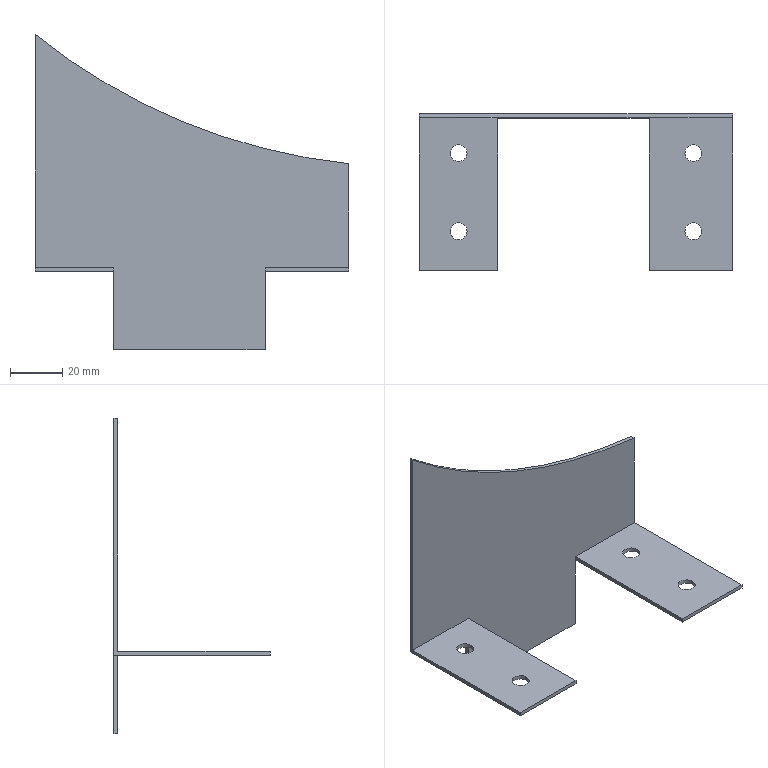Part | STEP file | 02-24 Battery support plate | 1 solid | 24 faces | box 120 x 60 x 120.818 mm | volume 18521 mm3 | plane 15 | cylinder 9 | commonest cylinder face diameters 6.5 x8 460 x1